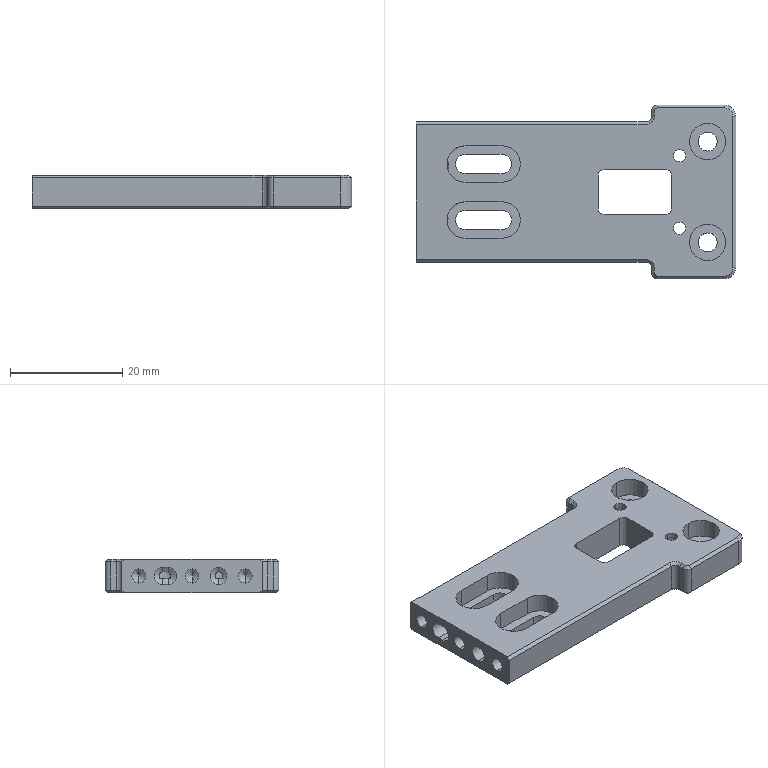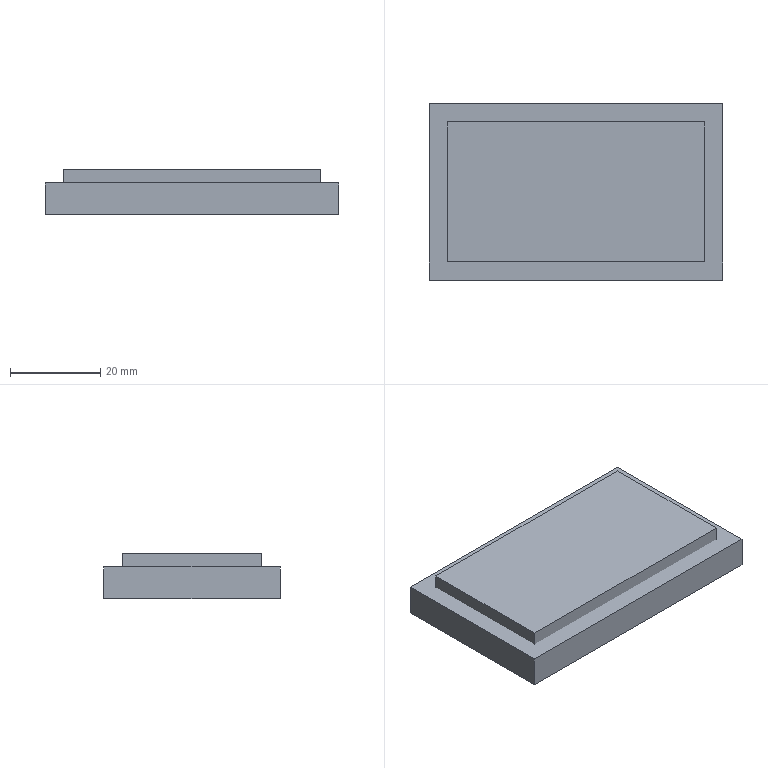CAM job | NX | 3+2 milling, drilling | part box 57 x 31 x 6 mm | stock box 65 x 39 x 10 mm
Tools:
number,name,description,diameter,corner_radius,flute_length,length,flutes
1,D50,Milling Tool-5 Parameters,50.0,0.0,50.0,75.0,2
7,D6A45,Milling Tool-5 Parameters,6.0,0.0,3.0,3.0,2
11,2.5ZT,Drilling Tool,2.5,0.0,35.0,50.0,2
10,D10,Milling Tool-5 Parameters,10.0,0.0,50.0,75.0,2
6,D6,Milling Tool-5 Parameters,6.0,0.0,50.0,75.0,2
4,D4,Milling Tool-5 Parameters,4.0,0.0,50.0,75.0,2
12,2.2ZT,Drilling Tool,2.2,0.0,35.0,50.0,2
13,3.4ZT,Drilling Tool,3.3,0.0,35.0,50.0,2
2,D2,Milling Tool-5 Parameters,2.0,0.0,50.0,75.0,2
Operations:
program,operation,operation_type,tool,method,geometry_group,spindle_rpm,surface_speed,feed_per_tooth,feed_cut,feed_plunge,cut_length_mm,path_length_mm,cut_time_min,machine_time_min
1-10-35-62毛胚-虎钳,FLOOR_WALL,VolumeBased25DMillingOperation,D50,METHOD,A,6500.0,1286.0,0.0962,1250.0,100.0,127.0,181.0,0.1016,0.107
1-10-35-62毛胚-虎钳,DRILLING_COPY_1,Operation,D6A45,METHOD,A,3000.0,56.0,0.0333,200.0,0.0,16.8,150.75,0.084,0.0974
1-10-35-62毛胚-虎钳,DRILLING_COPY_1_COPY_COPY_COPY_COPY_COPY_COPY_COPY,Operation,2.2ZT,METHOD,A,2000.0,15.0,0.0375,150.0,0.0,21.322,118.986,0.1421,0.1519
1-10-35-62毛胚-虎钳,DRILLING_COPY_1_COPY_COPY_COPY_COPY,Operation,3.4ZT,METHOD,A,2000.0,21.0,0.0375,150.0,0.0,20.983,123.214,0.1399,0.1501
1-10-35-62毛胚-虎钳,ADAPTIVE_MILLING,CavityMilling,D10,METHOD,A,7000.0,219.0,0.2143,3000.0,1000.0,1841.202,1907.202,0.6157,0.6223
1-10-35-62毛胚-虎钳,ZLEVEL_PROFILE_COPY,ZLevelMilling,D6,METHOD,A,7000.0,219.0,0.2143,3000.0,1000.0,308.791,371.791,0.1271,0.1334
1-10-35-62毛胚-虎钳,ZLEVEL_PROFILE_COPY_1_COPY,ZLevelMilling,D6,METHOD,A,7000.0,87.0,0.1071,1500.0,1000.0,183.58,437.829,0.1385,0.1639
1-10-35-62毛胚-虎钳,ZLEVEL_PROFILE_COPY_1,ZLevelMilling,D4,METHOD,A,7000.0,87.0,0.1071,1500.0,1000.0,421.742,1024.298,0.3142,0.3744
1-10-35-62毛胚-虎钳,ZLEVEL_PROFILE_COPY_COPY,ZLevelMilling,D4,METHOD,A,7000.0,87.0,0.1,1400.0,1000.0,605.482,735.323,0.452,0.4649
1-10-35-62毛胚-虎钳,ZLEVEL_PROFILE_COPY_COPY_1_COPY_COPY_COPY_1,ZLevelMilling,D4,METHOD,A,7000.0,219.0,0.0714,1000.0,100.0,212.827,395.867,0.2128,0.2311
1-10-35-62毛胚-虎钳,HOLE_MILLING,CylinderMilling,D4,METHOD,A,7000.0,131.0,0.1071,1500.0,100.0,227.914,371.714,0.1519,0.1663
1-10-35-62毛胚-虎钳,ZLEVEL_PROFILE_COPY_COPY_COPY,ZLevelMilling,D2,METHOD,A,7000.0,65.0,0.0857,1200.0,1000.0,713.857,857.295,0.6054,0.6197
1-10-35-62毛胚-虎钳,ZLEVEL_PROFILE_COPY_1_COPY_1,ZLevelMilling,D2,METHOD,A,7000.0,43.0,0.0786,1100.0,1000.0,887.847,1759.925,0.8192,0.9064
1-10-35-62毛胚-虎钳,ZLEVEL_PROFILE_COPY_1_COPY_COPY_COPY_COPY_2_COPY_COPY_1,ZLevelMilling,D6A45,METHOD,A,7000.0,131.0,0.0714,1000.0,1000.0,301.129,827.147,0.3011,0.3537
2-10-35-62毛胚-虎钳,FLOOR_WALL_COPY,VolumeBased25DMillingOperation,D50,METHOD,B,6500.0,1286.0,0.0962,1250.0,100.0,476.0,1019.001,0.3808,0.4351
2-10-35-62毛胚-虎钳,HOLE_MILLING_COPY,CylinderMilling,D2,METHOD,B,7000.0,43.0,0.0786,1100.0,100.0,216.119,358.119,0.1965,0.2107
2-10-35-62毛胚-虎钳,ZLEVEL_PROFILE_COPY_1_COPY_COPY_COPY_COPY_2_COPY_COPY_1_COPY,ZLevelMilling,D6A45,METHOD,B,7000.0,131.0,0.0714,1000.0,1000.0,278.531,952.415,0.2785,0.3459
2-10-35-62毛胚-虎钳,刀补5,CylinderMilling,D2,METHOD,B,7000.0,43.0,0.0607,850.0,100.0,42.285,184.286,0.0497,0.0639
3-10-35-62毛胚-虎钳,DRILLING_COPY_1_COPY_1,Operation,D6A45,METHOD,C,3000.0,56.0,0.0333,200.0,0.0,23.0,140.485,0.115,0.1267
3-10-35-62毛胚-虎钳,DRILLING_COPY_1_COPY_COPY_COPY_COPY_COPY_COPY,Operation,2.5ZT,METHOD,C,2000.0,15.0,0.0375,150.0,0.0,51.165,196.815,0.3411,0.3557
3-10-35-62毛胚-虎钳,ZLEVEL_PROFILE,ZLevelMilling,D2,METHOD,C,7000.0,65.0,0.0786,1100.0,1000.0,309.534,444.555,0.2854,0.2989
3-10-35-62毛胚-虎钳,ZLEVEL_PROFILE_COPY_1_COPY_COPY_COPY_COPY_2_COPY_COPY_1_1_COPY_1,ZLevelMilling,D6A45,METHOD,C,7000.0,131.0,0.0714,1000.0,1000.0,21.182,358.772,0.0212,0.0549
3-10-35-62毛胚-虎钳,刀补5.,ZLevelMilling,D2,METHOD,C,7000.0,65.0,0.0786,1100.0,1000.0,48.64,188.225,0.0444,0.0583